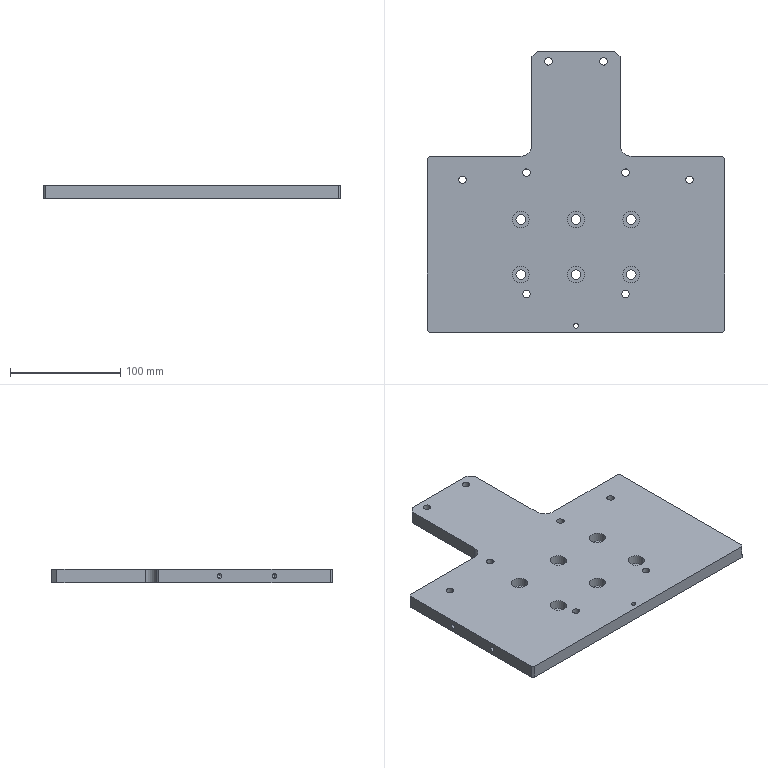Part | SolidWorks | features HoleWzd 7, Chamfer 2, Extrusion 1, Fillet 1, ICE 1, MirrorPattern 1 | 1 solid | 82 faces | box 270 x 255 x 12 mm | volume 594940 mm3 | cylinder 52 | plane 22 | cone 8 | commonest cylinder face diameters 6.8 x16 9 x12 15 x12 4.2 x10 20 x2